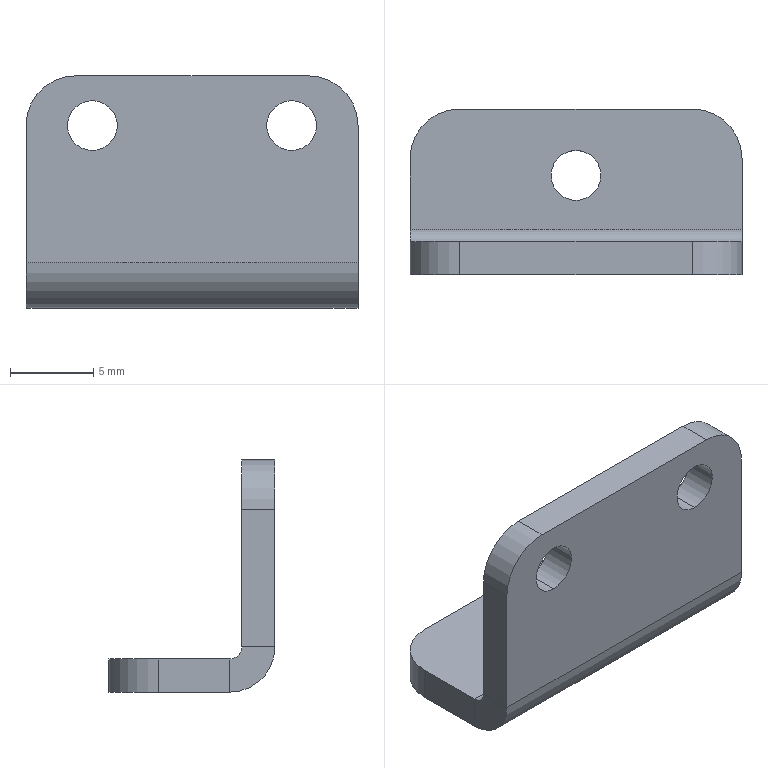Part | SolidWorks | features ICE 2, Fillet 1, FlatPattern 1, SMBaseFlange 1, SheetMetal 1 | 1 solid | 24 faces | box 20 x 10 x 14 mm | volume 792.323 mm3 | cylinder 12 | plane 12 | commonest cylinder face diameters 3 x6 6 x4 1.473 x1 5.473 x1
STEP:
#1=CARTESIAN_POINT('',(-1.5,4.,-14.));
#2=VERTEX_POINT('',#1);
#3=CARTESIAN_POINT('',(1.5,4.,-14.));
#4=VERTEX_POINT('',#3);
#5=CARTESIAN_POINT('',(0.,4.,-14.));
#6=DIRECTION('',(0.,0.,1.));
#7=DIRECTION('',(1.,0.,0.));
#8=AXIS2_PLACEMENT_3D('',#5,#6,#7);
#9=CIRCLE('',#8,1.5);
#10=EDGE_CURVE('',#2,#4,#9,.T.);
#11=ORIENTED_EDGE('',*,*,#10,.F.);
#12=CARTESIAN_POINT('',(-1.5,4.,-12.));
#13=VERTEX_POINT('',#12);
#14=CARTESIAN_POINT('',(-1.5,4.,-22.));
#15=DIRECTION('',(0.,0.,1.));
#16=VECTOR('',#15,1000.);
#17=LINE('',#14,#16);
#18=EDGE_CURVE('',#2,#13,#17,.T.);
#19=ORIENTED_EDGE('',*,*,#18,.T.);
#20=CARTESIAN_POINT('',(1.5,4.,-12.));
#21=VERTEX_POINT('',#20);
#22=CARTESIAN_POINT('',(0.,4.,-12.));
#23=DIRECTION('',(0.,0.,1.));
#24=DIRECTION('',(1.,0.,0.));
#25=AXIS2_PLACEMENT_3D('',#22,#23,#24);
#26=CIRCLE('',#25,1.5);
#27=EDGE_CURVE('',#13,#21,#26,.T.);
#28=ORIENTED_EDGE('',*,*,#27,.T.);
#29=CARTESIAN_POINT('',(1.5,4.,-22.));
#30=DIRECTION('',(0.,0.,1.));
#31=VECTOR('',#30,1000.);
#32=LINE('',#29,#31);
#33=EDGE_CURVE('',#4,#21,#32,.T.);
#34=ORIENTED_EDGE('',*,*,#33,.F.);
#35=EDGE_LOOP('',(#11,#19,#28,#34));
#36=FACE_OUTER_BOUND('',#35,.T.);
#37=CARTESIAN_POINT('',(0.,4.,-22.));
#38=DIRECTION('',(0.,0.,1.));
#39=DIRECTION('',(1.,0.,0.));
#40=AXIS2_PLACEMENT_3D('',#37,#38,#39);
#41=CYLINDRICAL_SURFACE('',#40,1.5);
#42=ADVANCED_FACE('',(#36),#41,.F.);
#43=CARTESIAN_POINT('',(6.,-2.,-4.5));
#44=VERTEX_POINT('',#43);
#45=CARTESIAN_POINT('',(6.,-2.,-1.5));
#46=VERTEX_POINT('',#45);
#47=CARTESIAN_POINT('',(6.,-2.,-3.));
#48=DIRECTION('',(0.,1.,0.));
#49=DIRECTION('',(0.,0.,1.));
#50=AXIS2_PLACEMENT_3D('',#47,#48,#49);
#51=CIRCLE('',#50,1.5);
#52=EDGE_CURVE('',#44,#46,#51,.T.);
#53=ORIENTED_EDGE('',*,*,#52,.F.);
#54=CARTESIAN_POINT('',(6.,0.,-4.5));
#55=VERTEX_POINT('',#54);
#56=CARTESIAN_POINT('',(6.,-10.,-4.5));
#57=DIRECTION('',(0.,1.,0.));
#58=VECTOR('',#57,1000.);
#59=LINE('',#56,#58);
#60=EDGE_CURVE('',#44,#55,#59,.T.);
#61=ORIENTED_EDGE('',*,*,#60,.T.);
#62=CARTESIAN_POINT('',(6.,0.,-1.5));
#63=VERTEX_POINT('',#62);
#64=CARTESIAN_POINT('',(6.,0.,-3.));
#65=DIRECTION('',(0.,1.,0.));
#66=DIRECTION('',(0.,0.,1.));
#67=AXIS2_PLACEMENT_3D('',#64,#65,#66);
#68=CIRCLE('',#67,1.5);
#69=EDGE_CURVE('',#55,#63,#68,.T.);
#70=ORIENTED_EDGE('',*,*,#69,.T.);
#71=CARTESIAN_POINT('',(6.,-10.,-1.5));
#72=DIRECTION('',(0.,1.,0.));
#73=VECTOR('',#72,1000.);
#74=LINE('',#71,#73);
#75=EDGE_CURVE('',#46,#63,#74,.T.);
#76=ORIENTED_EDGE('',*,*,#75,.F.);
#77=EDGE_LOOP('',(#53,#61,#70,#76));
#78=FACE_OUTER_BOUND('',#77,.T.);
#79=CARTESIAN_POINT('',(6.,-10.,-3.));
#80=DIRECTION('',(0.,1.,0.));
#81=DIRECTION('',(0.,0.,1.));
#82=AXIS2_PLACEMENT_3D('',#79,#80,#81);
#83=CYLINDRICAL_SURFACE('',#82,1.5);
#84=ADVANCED_FACE('',(#78),#83,.F.);
#85=CARTESIAN_POINT('',(-6.,-2.,-4.5));
#86=VERTEX_POINT('',#85);
#87=CARTESIAN_POINT('',(-6.,-2.,-1.5));
#88=VERTEX_POINT('',#87);
#89=CARTESIAN_POINT('',(-6.,-2.,-3.));
#90=DIRECTION('',(0.,1.,0.));
#91=DIRECTION('',(0.,0.,1.));
#92=AXIS2_PLACEMENT_3D('',#89,#90,#91);
#93=CIRCLE('',#92,1.5);
#94=EDGE_CURVE('',#86,#88,#93,.T.);
#95=ORIENTED_EDGE('',*,*,#94,.F.);
#96=CARTESIAN_POINT('',(-6.,0.,-4.5));
#97=VERTEX_POINT('',#96);
#98=CARTESIAN_POINT('',(-6.,-10.,-4.5));
#99=DIRECTION('',(0.,1.,0.));
#100=VECTOR('',#99,1000.);
#101=LINE('',#98,#100);
#102=EDGE_CURVE('',#86,#97,#101,.T.);
#103=ORIENTED_EDGE('',*,*,#102,.T.);
#104=CARTESIAN_POINT('',(-6.,0.,-1.5));
#105=VERTEX_POINT('',#104);
#106=CARTESIAN_POINT('',(-6.,0.,-3.));
#107=DIRECTION('',(0.,1.,0.));
#108=DIRECTION('',(0.,0.,1.));
#109=AXIS2_PLACEMENT_3D('',#106,#107,#108);
#110=CIRCLE('',#109,1.5);
#111=EDGE_CURVE('',#97,#105,#110,.T.);
#112=ORIENTED_EDGE('',*,*,#111,.T.);
#113=CARTESIAN_POINT('',(-6.,-10.,-1.5));
#114=DIRECTION('',(0.,1.,0.));
#115=VECTOR('',#114,1000.);
#116=LINE('',#113,#115);
#117=EDGE_CURVE('',#88,#105,#116,.T.);
#118=ORIENTED_EDGE('',*,*,#117,.F.);
#119=EDGE_LOOP('',(#95,#103,#112,#118));
#120=FACE_OUTER_BOUND('',#119,.T.);
#121=CARTESIAN_POINT('',(-6.,-10.,-3.));
#122=DIRECTION('',(0.,1.,0.));
#123=DIRECTION('',(0.,0.,1.));
#124=AXIS2_PLACEMENT_3D('',#121,#122,#123);
#125=CYLINDRICAL_SURFACE('',#124,1.5);
#126=ADVANCED_FACE('',(#120),#125,.F.);
#127=CARTESIAN_POINT('',(10.,0.7366,-12.));
#128=VERTEX_POINT('',#127);
#129=CARTESIAN_POINT('',(10.,0.7366,-14.));
#130=VERTEX_POINT('',#129);
#131=CARTESIAN_POINT('',(10.,0.7366,-12.));
#132=DIRECTION('',(0.,0.,-1.));
#133=VECTOR('',#132,1000.);
#134=LINE('',#131,#133);
#135=EDGE_CURVE('',#128,#130,#134,.T.);
#136=ORIENTED_EDGE('',*,*,#135,.F.);
#137=CARTESIAN_POINT('',(10.,0.,-11.263));
#138=VERTEX_POINT('',#137);
#139=CARTESIAN_POINT('',(10.,0.7366,-11.263));
#140=DIRECTION('',(1.,0.,0.));
#141=DIRECTION('',(0.,0.,1.));
#142=AXIS2_PLACEMENT_3D('',#139,#140,#141);
#143=CIRCLE('',#142,0.7366);
#144=EDGE_CURVE('',#138,#128,#143,.T.);
#145=ORIENTED_EDGE('',*,*,#144,.F.);
#146=CARTESIAN_POINT('',(10.,-2.,-11.263));
#147=VERTEX_POINT('',#146);
#148=CARTESIAN_POINT('',(10.,-2.,-11.263));
#149=DIRECTION('',(0.,1.,0.));
#150=VECTOR('',#149,1000.);
#151=LINE('',#148,#150);
#152=EDGE_CURVE('',#147,#138,#151,.T.);
#153=ORIENTED_EDGE('',*,*,#152,.F.);
#154=CARTESIAN_POINT('',(10.,0.7366,-11.263));
#155=DIRECTION('',(1.,0.,0.));
#156=DIRECTION('',(0.,0.,-1.));
#157=AXIS2_PLACEMENT_3D('',#154,#155,#156);
#158=CIRCLE('',#157,2.737);
#159=EDGE_CURVE('',#147,#130,#158,.T.);
#160=ORIENTED_EDGE('',*,*,#159,.T.);
#161=EDGE_LOOP('',(#136,#145,#153,#160));
#162=FACE_OUTER_BOUND('',#161,.T.);
#163=CARTESIAN_POINT('',(10.,0.7366,-12.));
#164=DIRECTION('',(1.,0.,0.));
#165=DIRECTION('',(0.,0.,-1.));
#166=AXIS2_PLACEMENT_3D('',#163,#164,#165);
#167=PLANE('',#166);
#168=ADVANCED_FACE('',(#162),#167,.T.);
#169=CARTESIAN_POINT('',(10.,5.,-14.));
#170=VERTEX_POINT('',#169);
#171=CARTESIAN_POINT('',(10.,0.,-14.));
#172=DIRECTION('',(0.,1.,0.));
#173=VECTOR('',#172,1000.);
#174=LINE('',#171,#173);
#175=EDGE_CURVE('',#130,#170,#174,.T.);
#176=ORIENTED_EDGE('',*,*,#175,.T.);
#177=CARTESIAN_POINT('',(10.,5.,-12.));
#178=VERTEX_POINT('',#177);
#179=CARTESIAN_POINT('',(10.,5.,-11.263));
#180=DIRECTION('',(0.,0.,1.));
#181=VECTOR('',#180,1000.);
#182=LINE('',#179,#181);
#183=EDGE_CURVE('',#170,#178,#182,.T.);
#184=ORIENTED_EDGE('',*,*,#183,.T.);
#185=CARTESIAN_POINT('',(10.,0.,-12.));
#186=DIRECTION('',(0.,1.,0.));
#187=VECTOR('',#186,1000.);
#188=LINE('',#185,#187);
#189=EDGE_CURVE('',#128,#178,#188,.T.);
#190=ORIENTED_EDGE('',*,*,#189,.F.);
#191=ORIENTED_EDGE('',*,*,#135,.T.);
#192=EDGE_LOOP('',(#176,#184,#190,#191));
#193=FACE_OUTER_BOUND('',#192,.T.);
#194=CARTESIAN_POINT('',(10.,-2.,-11.263));
#195=DIRECTION('',(1.,0.,0.));
#196=DIRECTION('',(0.,0.,-1.));
#197=AXIS2_PLACEMENT_3D('',#194,#195,#196);
#198=PLANE('',#197);
#199=ADVANCED_FACE('',(#193),#198,.T.);
#200=CARTESIAN_POINT('',(-10.,0.,-11.263));
#201=VERTEX_POINT('',#200);
#202=CARTESIAN_POINT('',(-10.,-2.,-11.263));
#203=VERTEX_POINT('',#202);
#204=CARTESIAN_POINT('',(-10.,0.,-11.263));
#205=DIRECTION('',(0.,-1.,0.));
#206=VECTOR('',#205,1000.);
#207=LINE('',#204,#206);
#208=EDGE_CURVE('',#201,#203,#207,.T.);
#209=ORIENTED_EDGE('',*,*,#208,.F.);
#210=CARTESIAN_POINT('',(-10.,0.7366,-12.));
#211=VERTEX_POINT('',#210);
#212=CARTESIAN_POINT('',(-10.,0.7366,-11.263));
#213=DIRECTION('',(1.,0.,0.));
#214=DIRECTION('',(0.,0.,1.));
#215=AXIS2_PLACEMENT_3D('',#212,#213,#214);
#216=CIRCLE('',#215,0.7366);
#217=EDGE_CURVE('',#201,#211,#216,.T.);
#218=ORIENTED_EDGE('',*,*,#217,.T.);
#219=CARTESIAN_POINT('',(-10.,0.7366,-14.));
#220=VERTEX_POINT('',#219);
#221=CARTESIAN_POINT('',(-10.,0.7366,-14.));
#222=DIRECTION('',(0.,0.,1.));
#223=VECTOR('',#222,1000.);
#224=LINE('',#221,#223);
#225=EDGE_CURVE('',#220,#211,#224,.T.);
#226=ORIENTED_EDGE('',*,*,#225,.F.);
#227=CARTESIAN_POINT('',(-10.,0.7366,-11.263));
#228=DIRECTION('',(1.,0.,0.));
#229=DIRECTION('',(0.,0.,-1.));
#230=AXIS2_PLACEMENT_3D('',#227,#228,#229);
#231=CIRCLE('',#230,2.737);
#232=EDGE_CURVE('',#203,#220,#231,.T.);
#233=ORIENTED_EDGE('',*,*,#232,.F.);
#234=EDGE_LOOP('',(#209,#218,#226,#233));
#235=FACE_OUTER_BOUND('',#234,.T.);
#236=CARTESIAN_POINT('',(-10.,0.,-11.263));
#237=DIRECTION('',(-1.,0.,0.));
#238=DIRECTION('',(0.,0.,1.));
#239=AXIS2_PLACEMENT_3D('',#236,#237,#238);
#240=PLANE('',#239);
#241=ADVANCED_FACE('',(#235),#240,.T.);
#242=CARTESIAN_POINT('',(-10.,-2.,-3.));
#243=VERTEX_POINT('',#242);
#244=CARTESIAN_POINT('',(-10.,-2.,0.));
#245=DIRECTION('',(0.,0.,-1.));
#246=VECTOR('',#245,1000.);
#247=LINE('',#244,#246);
#248=EDGE_CURVE('',#243,#203,#247,.T.);
#249=ORIENTED_EDGE('',*,*,#248,.F.);
#250=CARTESIAN_POINT('',(-10.,0.,-3.));
#251=VERTEX_POINT('',#250);
#252=CARTESIAN_POINT('',(-10.,0.7366,-3.));
#253=DIRECTION('',(0.,1.,0.));
#254=VECTOR('',#253,1000.);
#255=LINE('',#252,#254);
#256=EDGE_CURVE('',#243,#251,#255,.T.);
#257=ORIENTED_EDGE('',*,*,#256,.T.);
#258=CARTESIAN_POINT('',(-10.,0.,0.));
#259=DIRECTION('',(0.,0.,-1.));
#260=VECTOR('',#259,1000.);
#261=LINE('',#258,#260);
#262=EDGE_CURVE('',#251,#201,#261,.T.);
#263=ORIENTED_EDGE('',*,*,#262,.T.);
#264=ORIENTED_EDGE('',*,*,#208,.T.);
#265=EDGE_LOOP('',(#249,#257,#263,#264));
#266=FACE_OUTER_BOUND('',#265,.T.);
#267=CARTESIAN_POINT('',(-10.,0.7366,-14.));
#268=DIRECTION('',(-1.,0.,0.));
#269=DIRECTION('',(0.,0.,1.));
#270=AXIS2_PLACEMENT_3D('',#267,#268,#269);
#271=PLANE('',#270);
#272=ADVANCED_FACE('',(#266),#271,.T.);
#273=CARTESIAN_POINT('',(0.,4.,-14.));
#274=DIRECTION('',(0.,0.,1.));
#275=DIRECTION('',(1.,0.,0.));
#276=AXIS2_PLACEMENT_3D('',#273,#274,#275);
#277=CIRCLE('',#276,1.5);
#278=EDGE_CURVE('',#4,#2,#277,.T.);
#279=ORIENTED_EDGE('',*,*,#278,.T.);
#280=ORIENTED_EDGE('',*,*,#10,.T.);
#281=EDGE_LOOP('',(#279,#280));
#282=FACE_BOUND('',#281,.T.);
#283=CARTESIAN_POINT('',(-10.,5.,-14.));
#284=VERTEX_POINT('',#283);
#285=CARTESIAN_POINT('',(-10.,0.,-14.));
#286=DIRECTION('',(0.,1.,0.));
#287=VECTOR('',#286,1000.);
#288=LINE('',#285,#287);
#289=EDGE_CURVE('',#220,#284,#288,.T.);
#290=ORIENTED_EDGE('',*,*,#289,.T.);
#291=CARTESIAN_POINT('',(-7.,8.,-14.));
#292=VERTEX_POINT('',#291);
#293=CARTESIAN_POINT('',(-7.,5.,-14.));
#294=DIRECTION('',(0.,0.,-1.));
#295=DIRECTION('',(1.,0.,0.));
#296=AXIS2_PLACEMENT_3D('',#293,#294,#295);
#297=CIRCLE('',#296,3.);
#298=EDGE_CURVE('',#284,#292,#297,.T.);
#299=ORIENTED_EDGE('',*,*,#298,.T.);
#300=CARTESIAN_POINT('',(7.,8.,-14.));
#301=VERTEX_POINT('',#300);
#302=CARTESIAN_POINT('',(10.,8.,-14.));
#303=DIRECTION('',(-1.,0.,0.));
#304=VECTOR('',#303,1000.);
#305=LINE('',#302,#304);
#306=EDGE_CURVE('',#301,#292,#305,.T.);
#307=ORIENTED_EDGE('',*,*,#306,.F.);
#308=CARTESIAN_POINT('',(7.,5.,-14.));
#309=DIRECTION('',(0.,0.,-1.));
#310=DIRECTION('',(1.,0.,0.));
#311=AXIS2_PLACEMENT_3D('',#308,#309,#310);
#312=CIRCLE('',#311,3.);
#313=EDGE_CURVE('',#301,#170,#312,.T.);
#314=ORIENTED_EDGE('',*,*,#313,.T.);
#315=ORIENTED_EDGE('',*,*,#175,.F.);
#316=CARTESIAN_POINT('',(10.,0.7366,-14.));
#317=DIRECTION('',(-1.,0.,0.));
#318=VECTOR('',#317,1000.);
#319=LINE('',#316,#318);
#320=EDGE_CURVE('',#130,#220,#319,.T.);
#321=ORIENTED_EDGE('',*,*,#320,.T.);
#322=EDGE_LOOP('',(#290,#299,#307,#314,#315,#321));
#323=FACE_OUTER_BOUND('',#322,.T.);
#324=CARTESIAN_POINT('',(10.,0.,-14.));
#325=DIRECTION('',(0.,0.,1.));
#326=DIRECTION('',(1.,0.,0.));
#327=AXIS2_PLACEMENT_3D('',#324,#325,#326);
#328=PLANE('',#327);
#329=ADVANCED_FACE('',(#282,#323),#328,.F.);
#330=ORIENTED_EDGE('',*,*,#306,.T.);
#331=CARTESIAN_POINT('',(-7.,8.,-12.));
#332=VERTEX_POINT('',#331);
#333=CARTESIAN_POINT('',(-7.,8.,-12.));
#334=DIRECTION('',(0.,0.,1.));
#335=VECTOR('',#334,1000.);
#336=LINE('',#333,#335);
#337=EDGE_CURVE('',#292,#332,#336,.T.);
#338=ORIENTED_EDGE('',*,*,#337,.T.);
#339=CARTESIAN_POINT('',(7.,8.,-12.));
#340=VERTEX_POINT('',#339);
#341=CARTESIAN_POINT('',(10.,8.,-12.));
#342=DIRECTION('',(-1.,0.,0.));
#343=VECTOR('',#342,1000.);
#344=LINE('',#341,#343);
#345=EDGE_CURVE('',#340,#332,#344,.T.);
#346=ORIENTED_EDGE('',*,*,#345,.F.);
#347=CARTESIAN_POINT('',(7.,8.,-12.));
#348=DIRECTION('',(0.,0.,-1.));
#349=VECTOR('',#348,1000.);
#350=LINE('',#347,#349);
#351=EDGE_CURVE('',#340,#301,#350,.T.);
#352=ORIENTED_EDGE('',*,*,#351,.T.);
#353=EDGE_LOOP('',(#330,#338,#346,#352));
#354=FACE_OUTER_BOUND('',#353,.T.);
#355=CARTESIAN_POINT('',(10.,8.,-12.));
#356=DIRECTION('',(0.,1.,0.));
#357=DIRECTION('',(0.,0.,1.));
#358=AXIS2_PLACEMENT_3D('',#355,#356,#357);
#359=PLANE('',#358);
#360=ADVANCED_FACE('',(#354),#359,.T.);
#361=CARTESIAN_POINT('',(0.,4.,-12.));
#362=DIRECTION('',(0.,0.,1.));
#363=DIRECTION('',(1.,0.,0.));
#364=AXIS2_PLACEMENT_3D('',#361,#362,#363);
#365=CIRCLE('',#364,1.5);
#366=EDGE_CURVE('',#21,#13,#365,.T.);
#367=ORIENTED_EDGE('',*,*,#366,.F.);
#368=ORIENTED_EDGE('',*,*,#27,.F.);
#369=EDGE_LOOP('',(#367,#368));
#370=FACE_BOUND('',#369,.T.);
#371=ORIENTED_EDGE('',*,*,#345,.T.);
#372=CARTESIAN_POINT('',(-10.,5.,-12.));
#373=VERTEX_POINT('',#372);
#374=CARTESIAN_POINT('',(-7.,5.,-12.));
#375=DIRECTION('',(0.,0.,1.));
#376=DIRECTION('',(1.,0.,0.));
#377=AXIS2_PLACEMENT_3D('',#374,#375,#376);
#378=CIRCLE('',#377,3.);
#379=EDGE_CURVE('',#332,#373,#378,.T.);
#380=ORIENTED_EDGE('',*,*,#379,.T.);
#381=CARTESIAN_POINT('',(-10.,0.,-12.));
#382=DIRECTION('',(0.,1.,0.));
#383=VECTOR('',#382,1000.);
#384=LINE('',#381,#383);
#385=EDGE_CURVE('',#211,#373,#384,.T.);
#386=ORIENTED_EDGE('',*,*,#385,.F.);
#387=CARTESIAN_POINT('',(10.,0.7366,-12.));
#388=DIRECTION('',(-1.,0.,0.));
#389=VECTOR('',#388,1000.);
#390=LINE('',#387,#389);
#391=EDGE_CURVE('',#128,#211,#390,.T.);
#392=ORIENTED_EDGE('',*,*,#391,.F.);
#393=ORIENTED_EDGE('',*,*,#189,.T.);
#394=CARTESIAN_POINT('',(7.,5.,-12.));
#395=DIRECTION('',(0.,0.,1.));
#396=DIRECTION('',(1.,0.,0.));
#397=AXIS2_PLACEMENT_3D('',#394,#395,#396);
#398=CIRCLE('',#397,3.);
#399=EDGE_CURVE('',#178,#340,#398,.T.);
#400=ORIENTED_EDGE('',*,*,#399,.T.);
#401=EDGE_LOOP('',(#371,#380,#386,#392,#393,#400));
#402=FACE_OUTER_BOUND('',#401,.T.);
#403=CARTESIAN_POINT('',(10.,0.,-12.));
#404=DIRECTION('',(0.,0.,1.));
#405=DIRECTION('',(1.,0.,0.));
#406=AXIS2_PLACEMENT_3D('',#403,#404,#405);
#407=PLANE('',#406);
#408=ADVANCED_FACE('',(#370,#402),#407,.T.);
#409=ORIENTED_EDGE('',*,*,#217,.F.);
#410=CARTESIAN_POINT('',(10.,0.,-11.263));
#411=DIRECTION('',(-1.,0.,0.));
#412=VECTOR('',#411,1000.);
#413=LINE('',#410,#412);
#414=EDGE_CURVE('',#138,#201,#413,.T.);
#415=ORIENTED_EDGE('',*,*,#414,.F.);
#416=ORIENTED_EDGE('',*,*,#144,.T.);
#417=ORIENTED_EDGE('',*,*,#391,.T.);
#418=EDGE_LOOP('',(#409,#415,#416,#417));
#419=FACE_OUTER_BOUND('',#418,.T.);
#420=CARTESIAN_POINT('',(10.,0.7366,-11.263));
#421=DIRECTION('',(-1.,0.,0.));
#422=DIRECTION('',(0.,0.,1.));
#423=AXIS2_PLACEMENT_3D('',#420,#421,#422);
#424=CYLINDRICAL_SURFACE('',#423,0.7366);
#425=ADVANCED_FACE('',(#419),#424,.F.);
#426=CARTESIAN_POINT('',(6.,0.,-3.));
#427=DIRECTION('',(0.,1.,0.));
#428=DIRECTION('',(0.,0.,1.));
#429=AXIS2_PLACEMENT_3D('',#426,#427,#428);
#430=CIRCLE('',#429,1.5);
#431=EDGE_CURVE('',#63,#55,#430,.T.);
#432=ORIENTED_EDGE('',*,*,#431,.F.);
#433=ORIENTED_EDGE('',*,*,#69,.F.);
#434=EDGE_LOOP('',(#432,#433));
#435=FACE_BOUND('',#434,.T.);
#436=CARTESIAN_POINT('',(-6.,0.,-3.));
#437=DIRECTION('',(0.,1.,0.));
#438=DIRECTION('',(0.,0.,1.));
#439=AXIS2_PLACEMENT_3D('',#436,#437,#438);
#440=CIRCLE('',#439,1.5);
#441=EDGE_CURVE('',#105,#97,#440,.T.);
#442=ORIENTED_EDGE('',*,*,#441,.F.);
#443=ORIENTED_EDGE('',*,*,#111,.F.);
#444=EDGE_LOOP('',(#442,#443));
#445=FACE_BOUND('',#444,.T.);
#446=ORIENTED_EDGE('',*,*,#262,.F.);
#447=CARTESIAN_POINT('',(-7.,0.,0.));
#448=VERTEX_POINT('',#447);
#449=CARTESIAN_POINT('',(-7.,0.,-3.));
#450=DIRECTION('',(0.,1.,0.));
#451=DIRECTION('',(0.,0.,1.));
#452=AXIS2_PLACEMENT_3D('',#449,#450,#451);
#453=CIRCLE('',#452,3.);
#454=EDGE_CURVE('',#251,#448,#453,.T.);
#455=ORIENTED_EDGE('',*,*,#454,.T.);
#456=CARTESIAN_POINT('',(7.,0.,0.));
#457=VERTEX_POINT('',#456);
#458=CARTESIAN_POINT('',(10.,0.,0.));
#459=DIRECTION('',(-1.,0.,0.));
#460=VECTOR('',#459,1000.);
#461=LINE('',#458,#460);
#462=EDGE_CURVE('',#457,#448,#461,.T.);
#463=ORIENTED_EDGE('',*,*,#462,.F.);
#464=CARTESIAN_POINT('',(10.,0.,-3.));
#465=VERTEX_POINT('',#464);
#466=CARTESIAN_POINT('',(7.,0.,-3.));
#467=DIRECTION('',(0.,1.,0.));
#468=DIRECTION('',(0.,0.,1.));
#469=AXIS2_PLACEMENT_3D('',#466,#467,#468);
#470=CIRCLE('',#469,3.);
#471=EDGE_CURVE('',#457,#465,#470,.T.);
#472=ORIENTED_EDGE('',*,*,#471,.T.);
#473=CARTESIAN_POINT('',(10.,0.,0.));
#474=DIRECTION('',(0.,0.,-1.));
#475=VECTOR('',#474,1000.);
#476=LINE('',#473,#475);
#477=EDGE_CURVE('',#465,#138,#476,.T.);
#478=ORIENTED_EDGE('',*,*,#477,.T.);
#479=ORIENTED_EDGE('',*,*,#414,.T.);
#480=EDGE_LOOP('',(#446,#455,#463,#472,#478,#479));
#481=FACE_OUTER_BOUND('',#480,.T.);
#482=CARTESIAN_POINT('',(10.,0.,0.));
#483=DIRECTION('',(0.,1.,0.));
#484=DIRECTION('',(0.,0.,1.));
#485=AXIS2_PLACEMENT_3D('',#482,#483,#484);
#486=PLANE('',#485);
#487=ADVANCED_FACE('',(#435,#445,#481),#486,.T.);
#488=ORIENTED_EDGE('',*,*,#462,.T.);
#489=CARTESIAN_POINT('',(-7.,-2.,0.));
#490=VERTEX_POINT('',#489);
#491=CARTESIAN_POINT('',(-7.,-2.,0.));
#492=DIRECTION('',(0.,-1.,0.));
#493=VECTOR('',#492,1000.);
#494=LINE('',#491,#493);
#495=EDGE_CURVE('',#448,#490,#494,.T.);
#496=ORIENTED_EDGE('',*,*,#495,.T.);
#497=CARTESIAN_POINT('',(7.,-2.,0.));
#498=VERTEX_POINT('',#497);
#499=CARTESIAN_POINT('',(10.,-2.,0.));
#500=DIRECTION('',(-1.,0.,0.));
#501=VECTOR('',#500,1000.);
#502=LINE('',#499,#501);
#503=EDGE_CURVE('',#498,#490,#502,.T.);
#504=ORIENTED_EDGE('',*,*,#503,.F.);
#505=CARTESIAN_POINT('',(7.,0.,0.));
#506=DIRECTION('',(0.,1.,0.));
#507=VECTOR('',#506,1000.);
#508=LINE('',#505,#507);
#509=EDGE_CURVE('',#498,#457,#508,.T.);
#510=ORIENTED_EDGE('',*,*,#509,.T.);
#511=EDGE_LOOP('',(#488,#496,#504,#510));
#512=FACE_OUTER_BOUND('',#511,.T.);
#513=CARTESIAN_POINT('',(10.,-2.,0.));
#514=DIRECTION('',(0.,0.,1.));
#515=DIRECTION('',(1.,0.,0.));
#516=AXIS2_PLACEMENT_3D('',#513,#514,#515);
#517=PLANE('',#516);
#518=ADVANCED_FACE('',(#512),#517,.T.);
#519=CARTESIAN_POINT('',(6.,-2.,-3.));
#520=DIRECTION('',(0.,1.,0.));
#521=DIRECTION('',(0.,0.,1.));
#522=AXIS2_PLACEMENT_3D('',#519,#520,#521);
#523=CIRCLE('',#522,1.5);
#524=EDGE_CURVE('',#46,#44,#523,.T.);
#525=ORIENTED_EDGE('',*,*,#524,.T.);
#526=ORIENTED_EDGE('',*,*,#52,.T.);
#527=EDGE_LOOP('',(#525,#526));
#528=FACE_BOUND('',#527,.T.);
#529=CARTESIAN_POINT('',(-6.,-2.,-3.));
#530=DIRECTION('',(0.,1.,0.));
#531=DIRECTION('',(0.,0.,1.));
#532=AXIS2_PLACEMENT_3D('',#529,#530,#531);
#533=CIRCLE('',#532,1.5);
#534=EDGE_CURVE('',#88,#86,#533,.T.);
#535=ORIENTED_EDGE('',*,*,#534,.T.);
#536=ORIENTED_EDGE('',*,*,#94,.T.);
#537=EDGE_LOOP('',(#535,#536));
#538=FACE_BOUND('',#537,.T.);
#539=ORIENTED_EDGE('',*,*,#503,.T.);
#540=CARTESIAN_POINT('',(-7.,-2.,-3.));
#541=DIRECTION('',(0.,-1.,0.));
#542=DIRECTION('',(0.,0.,1.));
#543=AXIS2_PLACEMENT_3D('',#540,#541,#542);
#544=CIRCLE('',#543,3.);
#545=EDGE_CURVE('',#490,#243,#544,.T.);
#546=ORIENTED_EDGE('',*,*,#545,.T.);
#547=ORIENTED_EDGE('',*,*,#248,.T.);
#548=CARTESIAN_POINT('',(10.,-2.,-11.263));
#549=DIRECTION('',(-1.,0.,0.));
#550=VECTOR('',#549,1000.);
#551=LINE('',#548,#550);
#552=EDGE_CURVE('',#147,#203,#551,.T.);
#553=ORIENTED_EDGE('',*,*,#552,.F.);
#554=CARTESIAN_POINT('',(10.,-2.,-3.));
#555=VERTEX_POINT('',#554);
#556=CARTESIAN_POINT('',(10.,-2.,0.));
#557=DIRECTION('',(0.,0.,-1.));
#558=VECTOR('',#557,1000.);
#559=LINE('',#556,#558);
#560=EDGE_CURVE('',#555,#147,#559,.T.);
#561=ORIENTED_EDGE('',*,*,#560,.F.);
#562=CARTESIAN_POINT('',(7.,-2.,-3.));
#563=DIRECTION('',(0.,-1.,0.));
#564=DIRECTION('',(0.,0.,1.));
#565=AXIS2_PLACEMENT_3D('',#562,#563,#564);
#566=CIRCLE('',#565,3.);
#567=EDGE_CURVE('',#555,#498,#566,.T.);
#568=ORIENTED_EDGE('',*,*,#567,.T.);
#569=EDGE_LOOP('',(#539,#546,#547,#553,#561,#568));
#570=FACE_OUTER_BOUND('',#569,.T.);
#571=CARTESIAN_POINT('',(10.,-2.,0.));
#572=DIRECTION('',(0.,1.,0.));
#573=DIRECTION('',(0.,0.,1.));
#574=AXIS2_PLACEMENT_3D('',#571,#572,#573);
#575=PLANE('',#574);
#576=ADVANCED_FACE('',(#528,#538,#570),#575,.F.);
#577=ORIENTED_EDGE('',*,*,#232,.T.);
#578=ORIENTED_EDGE('',*,*,#320,.F.);
#579=ORIENTED_EDGE('',*,*,#159,.F.);
#580=ORIENTED_EDGE('',*,*,#552,.T.);
#581=EDGE_LOOP('',(#577,#578,#579,#580));
#582=FACE_OUTER_BOUND('',#581,.T.);
#583=CARTESIAN_POINT('',(10.,0.7366,-11.263));
#584=DIRECTION('',(-1.,0.,0.));
#585=DIRECTION('',(0.,0.,1.));
#586=AXIS2_PLACEMENT_3D('',#583,#584,#585);
#587=CYLINDRICAL_SURFACE('',#586,2.737);
#588=ADVANCED_FACE('',(#582),#587,.T.);
#589=ORIENTED_EDGE('',*,*,#477,.F.);
#590=CARTESIAN_POINT('',(10.,-2.,-3.));
#591=DIRECTION('',(0.,-1.,0.));
#592=VECTOR('',#591,1000.);
#593=LINE('',#590,#592);
#594=EDGE_CURVE('',#465,#555,#593,.T.);
#595=ORIENTED_EDGE('',*,*,#594,.T.);
#596=ORIENTED_EDGE('',*,*,#560,.T.);
#597=ORIENTED_EDGE('',*,*,#152,.T.);
#598=EDGE_LOOP('',(#589,#595,#596,#597));
#599=FACE_OUTER_BOUND('',#598,.T.);
#600=CARTESIAN_POINT('',(10.,0.7366,-11.263));
#601=DIRECTION('',(-1.,0.,0.));
#602=DIRECTION('',(0.,0.,1.));
#603=AXIS2_PLACEMENT_3D('',#600,#601,#602);
#604=PLANE('',#603);
#605=ADVANCED_FACE('',(#599),#604,.F.);
#606=ORIENTED_EDGE('',*,*,#385,.T.);
#607=CARTESIAN_POINT('',(-10.,5.,-11.263));
#608=DIRECTION('',(0.,0.,-1.));
#609=VECTOR('',#608,1000.);
#610=LINE('',#607,#609);
#611=EDGE_CURVE('',#373,#284,#610,.T.);
#612=ORIENTED_EDGE('',*,*,#611,.T.);
#613=ORIENTED_EDGE('',*,*,#289,.F.);
#614=ORIENTED_EDGE('',*,*,#225,.T.);
#615=EDGE_LOOP('',(#606,#612,#613,#614));
#616=FACE_OUTER_BOUND('',#615,.T.);
#617=CARTESIAN_POINT('',(-10.,0.7366,-11.263));
#618=DIRECTION('',(-1.,0.,0.));
#619=DIRECTION('',(0.,0.,1.));
#620=AXIS2_PLACEMENT_3D('',#617,#618,#619);
#621=PLANE('',#620);
#622=ADVANCED_FACE('',(#616),#621,.T.);
#623=ORIENTED_EDGE('',*,*,#379,.F.);
#624=ORIENTED_EDGE('',*,*,#337,.F.);
#625=ORIENTED_EDGE('',*,*,#298,.F.);
#626=ORIENTED_EDGE('',*,*,#611,.F.);
#627=EDGE_LOOP('',(#623,#624,#625,#626));
#628=FACE_OUTER_BOUND('',#627,.T.);
#629=CARTESIAN_POINT('',(-7.,5.,-11.263));
#630=DIRECTION('',(0.,0.,-1.));
#631=DIRECTION('',(-1.,0.,0.));
#632=AXIS2_PLACEMENT_3D('',#629,#630,#631);
#633=CYLINDRICAL_SURFACE('',#632,3.);
#634=ADVANCED_FACE('',(#628),#633,.T.);
#635=ORIENTED_EDGE('',*,*,#545,.F.);
#636=ORIENTED_EDGE('',*,*,#495,.F.);
#637=ORIENTED_EDGE('',*,*,#454,.F.);
#638=ORIENTED_EDGE('',*,*,#256,.F.);
#639=EDGE_LOOP('',(#635,#636,#637,#638));
#640=FACE_OUTER_BOUND('',#639,.T.);
#641=CARTESIAN_POINT('',(-7.,0.7366,-3.));
#642=DIRECTION('',(0.,1.,0.));
#643=DIRECTION('',(0.,0.,1.));
#644=AXIS2_PLACEMENT_3D('',#641,#642,#643);
#645=CYLINDRICAL_SURFACE('',#644,3.);
#646=ADVANCED_FACE('',(#640),#645,.T.);
#647=ORIENTED_EDGE('',*,*,#567,.F.);
#648=ORIENTED_EDGE('',*,*,#594,.F.);
#649=ORIENTED_EDGE('',*,*,#471,.F.);
#650=ORIENTED_EDGE('',*,*,#509,.F.);
#651=EDGE_LOOP('',(#647,#648,#649,#650));
#652=FACE_OUTER_BOUND('',#651,.T.);
#653=CARTESIAN_POINT('',(7.,-2.,-3.));
#654=DIRECTION('',(0.,-1.,0.));
#655=DIRECTION('',(0.,0.,-1.));
#656=AXIS2_PLACEMENT_3D('',#653,#654,#655);
#657=CYLINDRICAL_SURFACE('',#656,3.);
#658=ADVANCED_FACE('',(#652),#657,.T.);
#659=ORIENTED_EDGE('',*,*,#399,.F.);
#660=ORIENTED_EDGE('',*,*,#183,.F.);
#661=ORIENTED_EDGE('',*,*,#313,.F.);
#662=ORIENTED_EDGE('',*,*,#351,.F.);
#663=EDGE_LOOP('',(#659,#660,#661,#662));
#664=FACE_OUTER_BOUND('',#663,.T.);
#665=CARTESIAN_POINT('',(7.,5.,-12.));
#666=DIRECTION('',(0.,0.,-1.));
#667=DIRECTION('',(-1.,0.,0.));
#668=AXIS2_PLACEMENT_3D('',#665,#666,#667);
#669=CYLINDRICAL_SURFACE('',#668,3.);
#670=ADVANCED_FACE('',(#664),#669,.T.);
#671=ORIENTED_EDGE('',*,*,#102,.F.);
#672=ORIENTED_EDGE('',*,*,#534,.F.);
#673=ORIENTED_EDGE('',*,*,#117,.T.);
#674=ORIENTED_EDGE('',*,*,#441,.T.);
#675=EDGE_LOOP('',(#671,#672,#673,#674));
#676=FACE_OUTER_BOUND('',#675,.T.);
#677=CARTESIAN_POINT('',(-6.,-10.,-3.));
#678=DIRECTION('',(0.,1.,0.));
#679=DIRECTION('',(0.,0.,1.));
#680=AXIS2_PLACEMENT_3D('',#677,#678,#679);
#681=CYLINDRICAL_SURFACE('',#680,1.5);
#682=ADVANCED_FACE('',(#676),#681,.F.);
#683=ORIENTED_EDGE('',*,*,#60,.F.);
#684=ORIENTED_EDGE('',*,*,#524,.F.);
#685=ORIENTED_EDGE('',*,*,#75,.T.);
#686=ORIENTED_EDGE('',*,*,#431,.T.);
#687=EDGE_LOOP('',(#683,#684,#685,#686));
#688=FACE_OUTER_BOUND('',#687,.T.);
#689=CARTESIAN_POINT('',(6.,-10.,-3.));
#690=DIRECTION('',(0.,1.,0.));
#691=DIRECTION('',(0.,0.,1.));
#692=AXIS2_PLACEMENT_3D('',#689,#690,#691);
#693=CYLINDRICAL_SURFACE('',#692,1.5);
#694=ADVANCED_FACE('',(#688),#693,.F.);
#695=ORIENTED_EDGE('',*,*,#18,.F.);
#696=ORIENTED_EDGE('',*,*,#278,.F.);
#697=ORIENTED_EDGE('',*,*,#33,.T.);
#698=ORIENTED_EDGE('',*,*,#366,.T.);
#699=EDGE_LOOP('',(#695,#696,#697,#698));
#700=FACE_OUTER_BOUND('',#699,.T.);
#701=CARTESIAN_POINT('',(0.,4.,-22.));
#702=DIRECTION('',(0.,0.,1.));
#703=DIRECTION('',(1.,0.,0.));
#704=AXIS2_PLACEMENT_3D('',#701,#702,#703);
#705=CYLINDRICAL_SURFACE('',#704,1.5);
#706=ADVANCED_FACE('',(#700),#705,.F.);
#707=CLOSED_SHELL('',(#42,#84,#126,#168,#199,#241,#272,#329,#360,#408,#425,#487,#518,#576,#588,#605,#622,#634,#646,#658,#670,#682,#694,#706));
#708=MANIFOLD_SOLID_BREP('',#707);
#709=CARTESIAN_POINT('',(0.,0.,0.));
#710=DIRECTION('',(0.,0.,1.));
#711=DIRECTION('',(1.,0.,0.));
#712=AXIS2_PLACEMENT_3D('',#709,#710,#711);
#713=(LENGTH_UNIT()NAMED_UNIT(*)SI_UNIT(.MILLI.,.METRE.));
#714=UNCERTAINTY_MEASURE_WITH_UNIT(LENGTH_MEASURE(0.00001),#713,'','');
#715=(NAMED_UNIT(*)PLANE_ANGLE_UNIT()SI_UNIT($,.RADIAN.));
#716=(NAMED_UNIT(*)SI_UNIT($,.STERADIAN.)SOLID_ANGLE_UNIT());
#717=(GEOMETRIC_REPRESENTATION_CONTEXT(3)GLOBAL_UNCERTAINTY_ASSIGNED_CONTEXT((#714))GLOBAL_UNIT_ASSIGNED_CONTEXT((#713,#715,#716))REPRESENTATION_CONTEXT('',''));
#718=ADVANCED_BREP_SHAPE_REPRESENTATION('',(#708,#712),#717);